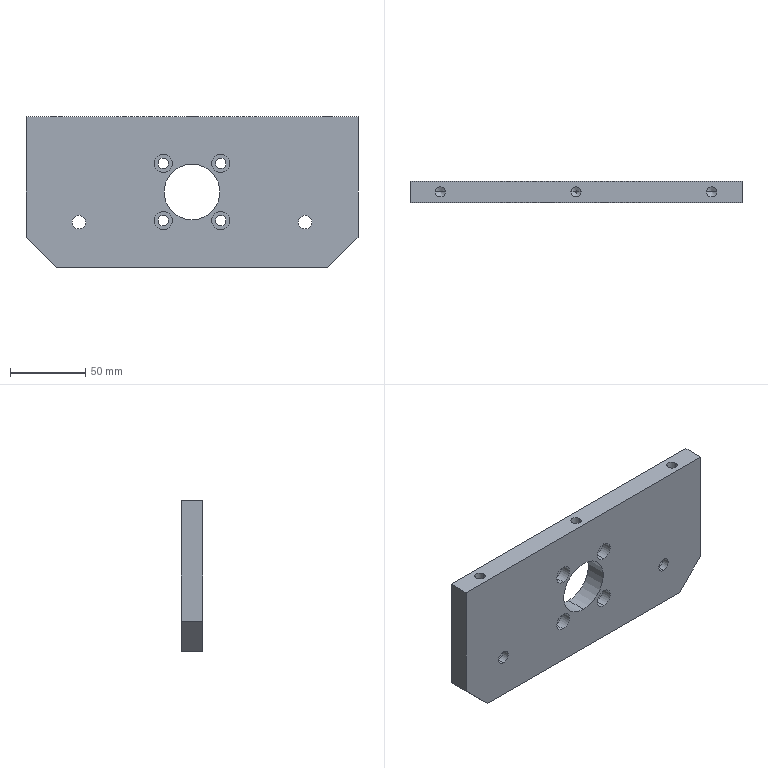Part | STEP file | fBY02F02M-00-08A | 1 solid | 52 faces | box 220 x 14 x 100 mm | volume 276380 mm3 | cylinder 32 | plane 14 | cone 6 | commonest cylinder face diameters 7 x8 12 x8 6.8 x6 9 x4 14 x4 37 x2